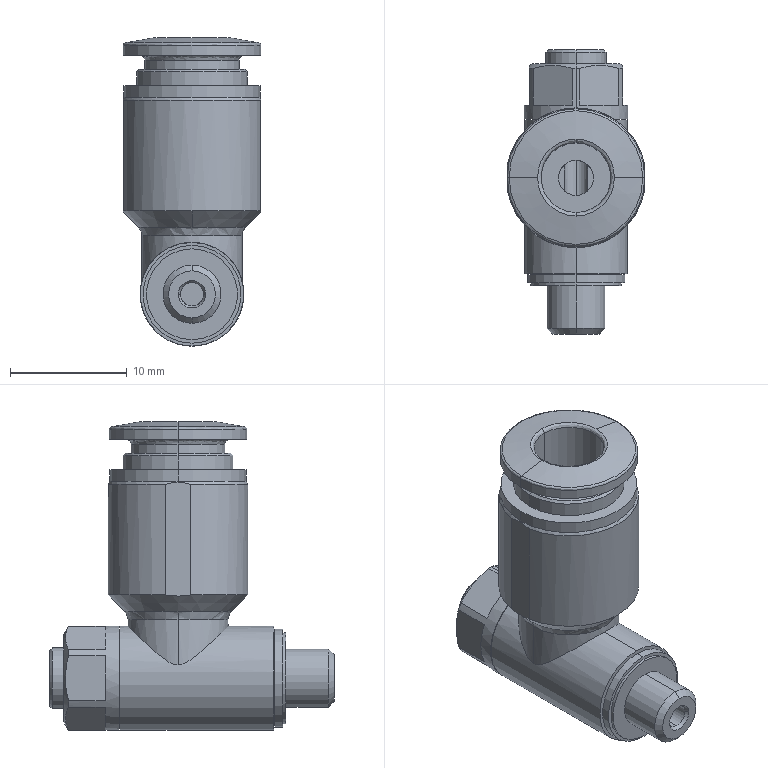Part | SolidWorks | features BaseBody 1 | 1 solid | 99 faces | box 11.8 x 24.4 x 26.45 mm | volume 2431 mm3 | plane 35 | cylinder 34 | cone 20 | spline 10 | commonest cylinder face diameters 8.9 x4 2 x2 3 x2 4.2 x2 5 x2 5.2 x2